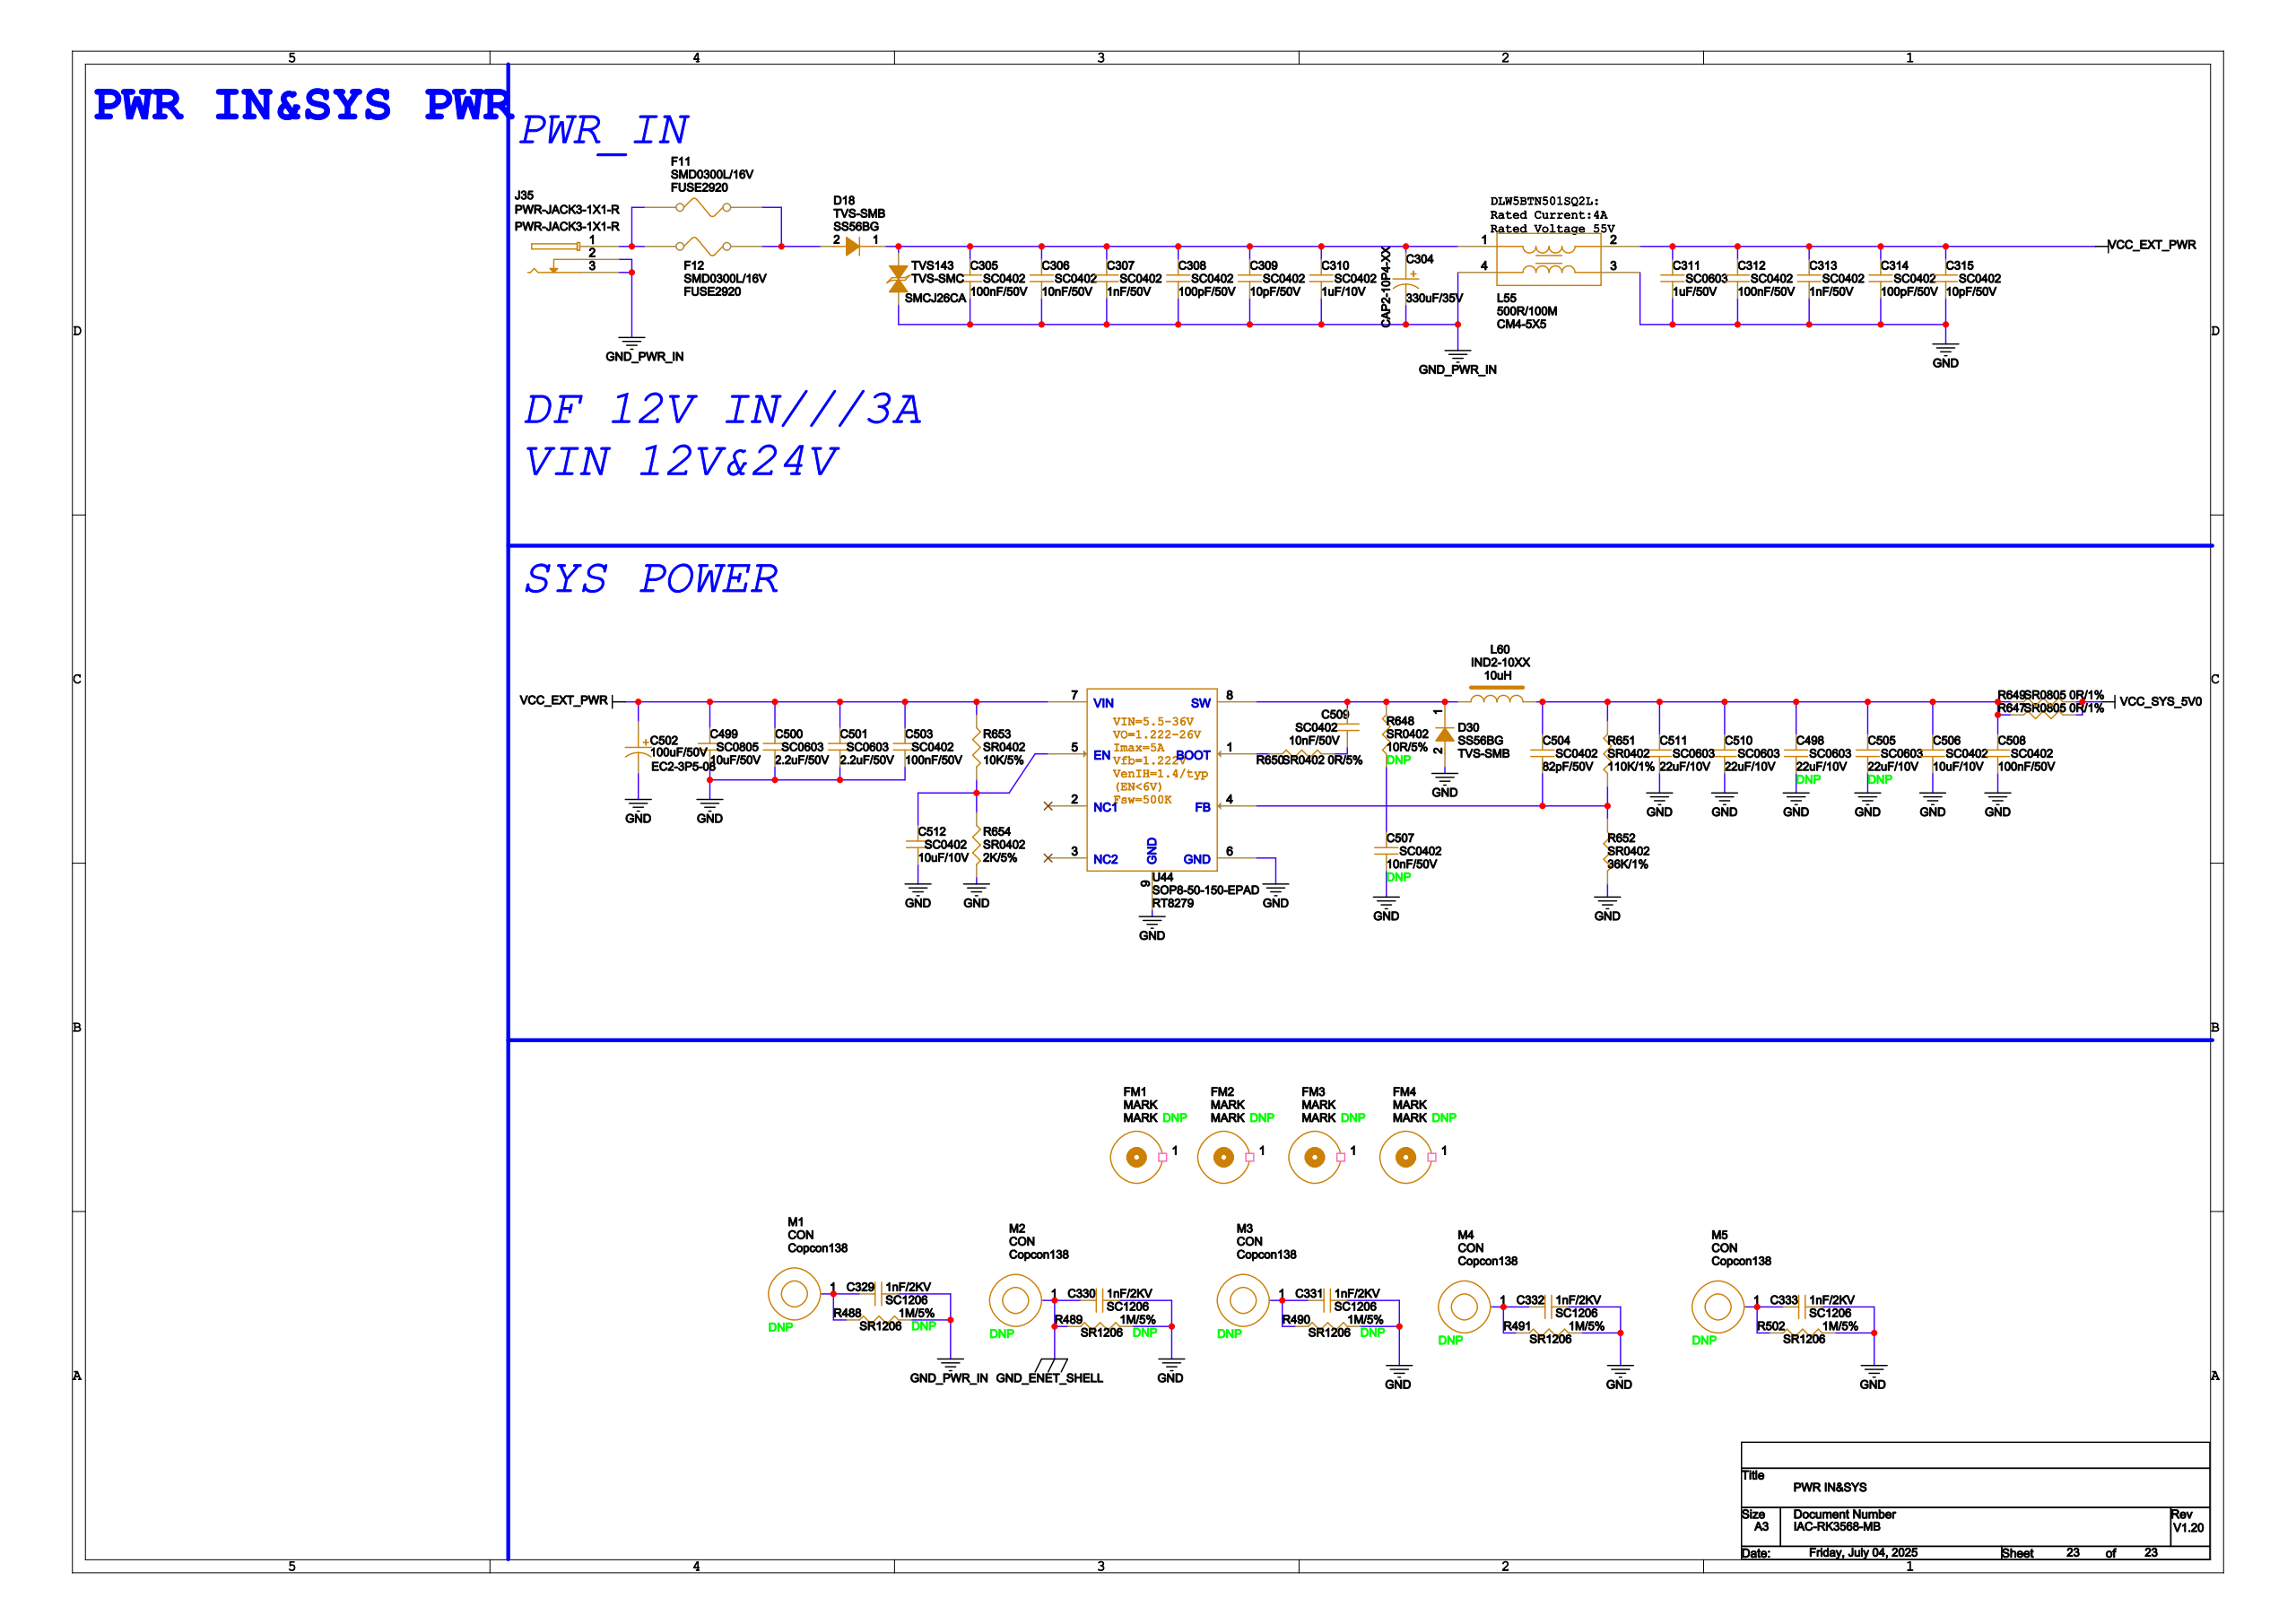Circuit board | Cadence Allegro | 1138 parts | 722 nets | one sheet of the schematic
Parts on this sheet (reference | value | footprint):
C304 | 330uF/35V | CAP2-10P4-XX
C305 | 100nF/50V | SC0402
C306 | 10nF/50V | SC0402
C307 | 1nF/50V | SC0402
C308 | 100pF/50V | SC0402
C309 | 10pF/50V | SC0402
C310 | 1uF/10V | SC0402
C311 | 1uF/50V | SC0603
C312 | 100nF/50V | SC0402
C313 | 1nF/50V | SC0402
C314 | 100pF/50V | SC0402
C315 | 10pF/50V | SC0402
C329 | 1nF/2KV | SC1206
C330 | 1nF/2KV | SC1206
C331 | 1nF/2KV | SC1206
C332 | 1nF/2KV | SC1206
C333 | 1nF/2KV | SC1206
C498 | 22uF/10V | SC0603
C499 | 10uF/50V | SC0805
C500 | 2.2uF/50V | SC0603
C501 | 2.2uF/50V | SC0603
C503 | 100nF/50V | SC0402
C504 | 82pF/50V | SC0402
C505 | 22uF/10V | SC0603
C506 | 10uF/10V | SC0402
C507 | 10nF/50V | SC0402
C508 | 100nF/50V | SC0402
C509 | 10nF/50V | SC0402
C510 | 22uF/10V | SC0603
C511 | 22uF/10V | SC0603
C512 | 10uF/10V | SC0402
D18 | SS56BG | TVS-SMB
D30 | SS56BG | TVS-SMB
F11 | SMD0300L/16V | FUSE2920
F12 | SMD0300L/16V | FUSE2920
J35 | PWR-JACK3-1X1-R | PWR-JACK3-1X1-R
L55 | 500R/100M | CM4-5X5
L60 | 10uH | IND2-10XX
M1 | CON | COPCON138
M2 | CON | COPCON138
M3 | CON | COPCON138
M4 | CON | COPCON138
M5 | CON | COPCON138
R488 | 1M/5% | SR1206
R489 | 1M/5% | SR1206
R490 | 1M/5% | SR1206
R491 | 1M/5% | SR1206
R502 | 1M/5% | SR1206
R648 | 10R/5% | SR0402
R651 | 110K/1% | SR0402
R652 | 36K/1% | SR0402
R653 | 10K/5% | SR0402
R654 | 2K/5% | SR0402
TVS143 | SMCJ26CA | TVS-SMC
U44 | RT8279 | SOP8-50-150-EPAD
Nets of these parts (net: part-pin ...):
N6659744: D18-2 F11-1 F12-1
N3626765: C304-1 C305-1 C306-1 C307-1 C308-1 C309-1 C310-1 D18-1 L55-1 TVS143-2
GND: C311-2 C312-2 C313-2 C314-2 C315-2 C330-2 C331-2 C332-2 C333-2 C498-2 C499-2 C500-2 C501-2 C503-2 C505-2 C506-2 C507-2 C508-2 C510-2 C511-2 C512-2 D30-2 L55-3 R489-2 R490-2 R491-2 R502-2 R652-2 R654-2 U44-6 U44-9
N16419759: C509-1 D30-1 L60-1 R648-2 U44-8
VCC_EXT_PWR: C311-1 C312-1 C313-1 C314-1 C315-1 C499-1 C500-1 C501-1 C503-1 L55-2 R653-1 U44-7
N16419767: C498-1 C504-1 C505-1 C506-1 C508-1 C510-1 C511-1 L60-2 R651-2
N16419803: C504-2 R651-1 R652-1 U44-4
N16420591: C512-1 R653-2 R654-1 U44-5
N16419959: C507-1 R648-1
GND_PWR_IN: C304-2 C305-2 C306-2 C307-2 C308-2 C309-2 C310-2 C329-2 J35-2 J35-3 L55-4 R488-2 TVS143-1
N16419799: U44-1
GND_ENET_SHELL: C330-1 M2-1 R489-1
N4118311: C329-1 M1-1 R488-1
N4118499: C331-1 M3-1 R490-1
N4118573: C332-1 M4-1 R491-1
N5031794: C333-1 M5-1 R502-1
N16419747: C509-2
N19683591: F11-2 F12-2 J35-1